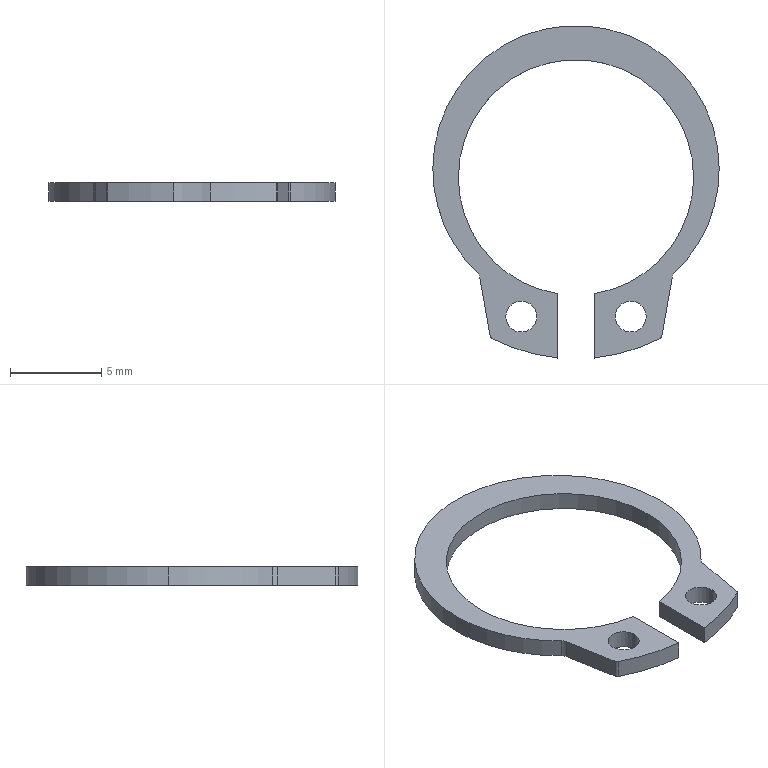Part | STEP file | circlips for shaft--type a large gb_GB_CONNECTING_PIECE_RING_RRA 14 | 1 solid | 22 faces | box 15.7 x 18.22 x 1 mm | volume 78.336 mm3 | cylinder 16 | plane 6 | commonest cylinder face diameters 1.7 x4 12.9 x3 15.7 x3 0.4 x2 1 x2 19.9 x2